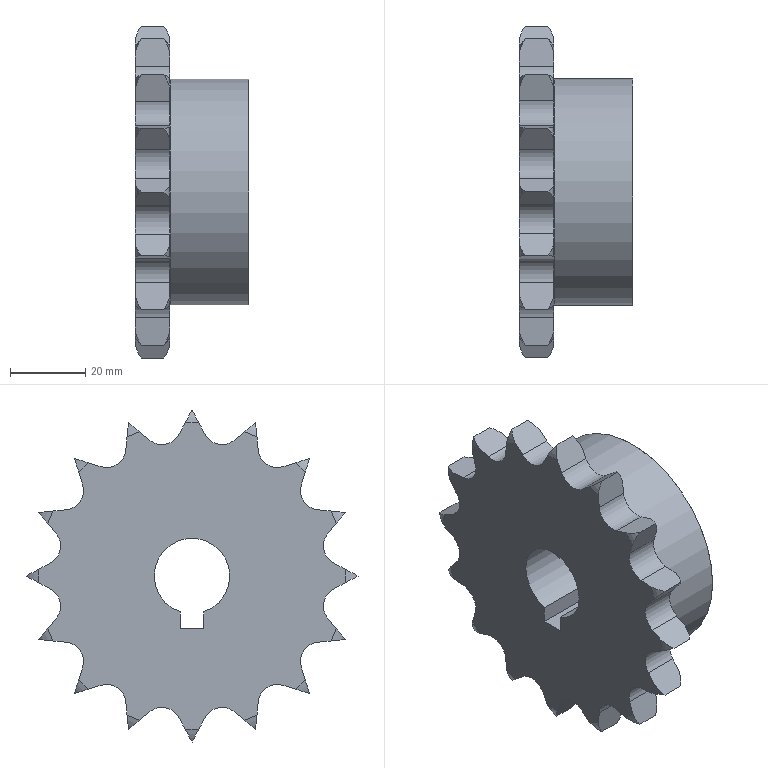Part | STEP file | 10B-1 z16_1 | 1 solid | 90 faces | box 30 x 88 x 88 mm | volume 91202 mm3 | plane 38 | torus 34 | cylinder 18 | commonest cylinder face diameters 10.16 x16 20 x1 60.14 x1